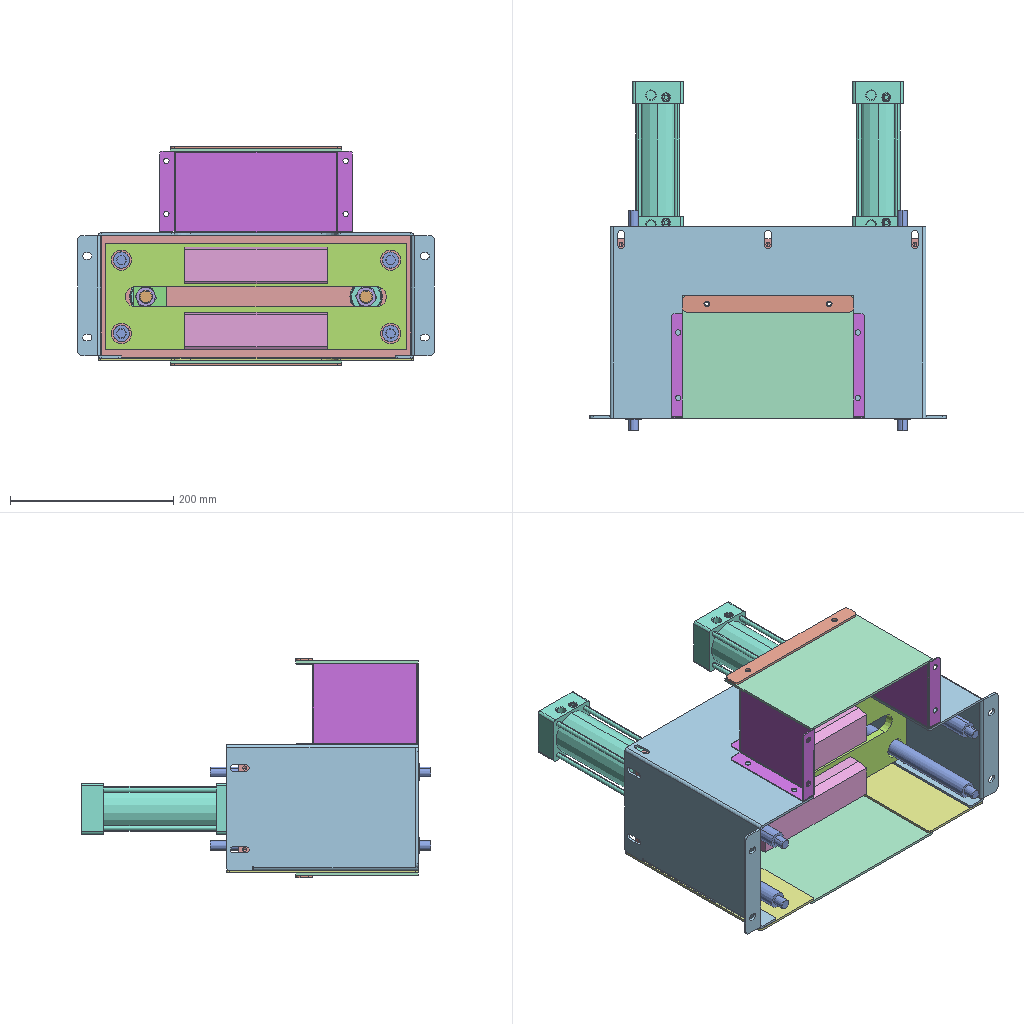Assembly | SolidWorks | 15 different items | 25 placed | box 437 x 428 x 269 mm
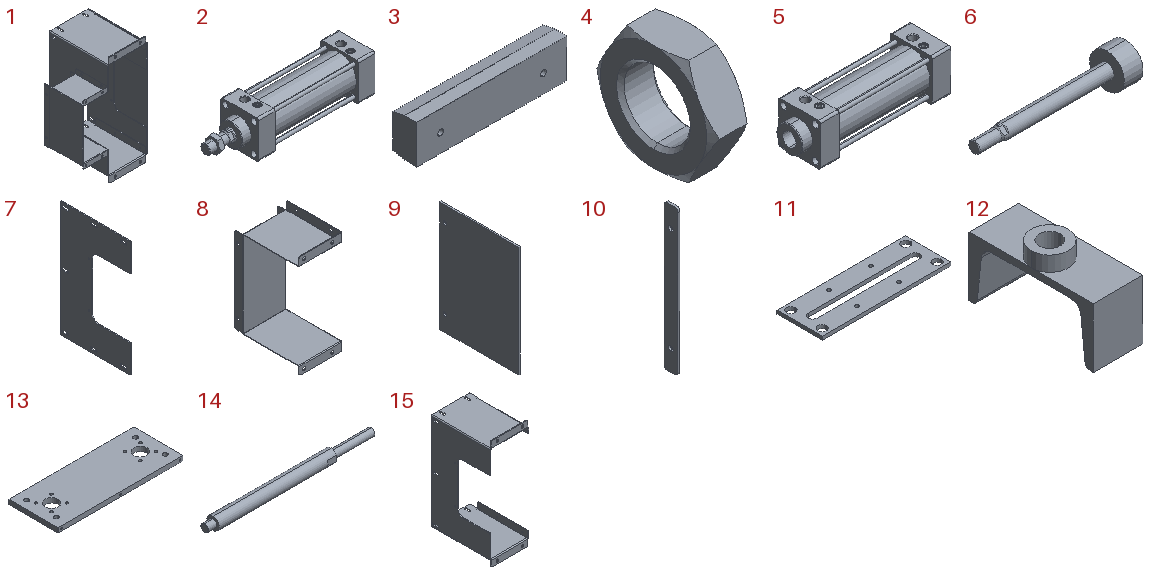Parts list (item | name | quantity | parent item | size | volume | features):
1 | (subassembly) | x1 | - | 269 x 235 x 437 mm | 927122 mm3 | features AEMSimFeature 1
2 | (subassembly) | x2 | - | 250 x 62 x 62 mm | 379695 mm3 | -
3 | - | x2 | - | 175 x 28 x 45 mm | 211666 mm3 | features Extrusion 1, HoleWzd 1, ICE 1
4 | - | x2 | in 2 | 8 x 26.558 x 23 mm | 2309 mm3 | features BaseBody 1
5 | - | x2 | in 2 | 208 x 62 x 62 mm | 269760 mm3 | features BaseBody 1
6 | - | x2 | in 2 | 217 x 49.5 x 49.5 mm | 107628 mm3 | features BaseBody 1
7 | - | x1 | in 1 | 3 x 235 x 387 mm | 191622 mm3 | features Fillet 3, FlatPattern 1, HoleWzd 1, ICE 1, SMBaseFlange 1, SheetMetal 1
8 | - | x1 | in 1 | 100 x 148.8 x 237.6 mm | 72757 mm3 | features HoleWzd 3, EdgeFlange 2, Fillet 2, FlatPattern 1, SMBaseFlange 1, SheetMetal 1
9 | - | x2 | in 1 | 3 x 150 x 210 mm | 94269 mm3 | features FlatPattern 1, HoleWzd 1, SMBaseFlange 1, SheetMetal 1
10 | - | x2 | in 1 | 3 x 20 x 210 mm | 12305 mm3 | features Fillet 1, FlatPattern 1, HoleWzd 1, SMBaseFlange 1, SheetMetal 1
11 | - | x1 | - | 370 x 130 x 10 mm | 379565 mm3 | features Extrusion 1, HoleWzd 1
12 | - | x1 | - | 40 x 100 x 60 mm | 55523 mm3 | features ICE 2, 3DProfileFeature 1, WeldMemberFeat 1, WeldmentFeature 1
13 | - | x1 | - | 380 x 150 x 14 mm | 746680 mm3 | features HoleWzd 6, 3DProfileFeature 2, Chamfer 1, Extrusion 1, ICE 1, LPattern 1
14 | - | x4 | - | 270 x 20 x 20 mm | 68758 mm3 | features ICE 2, Chamfer 1, Revolution 1
15 | - | x1 | in 1 | 154 x 235 x 437 mm | 449596 mm3 | features Fillet 4, ICE 4, EdgeFlange 3, HoleWzd 2, Cut 1, FlatPattern 1, SMBaseFlange 1, SheetMetal 1
Mates (type | each side: item.copy, entity, surface, feature):
In the top assembly
Coincident | 13.1 face plane Boss-Extrude1 | assembly face
Concentric | 13.1 face cylinder Cut-Extrude1 | assembly face
Concentric | 13.1 face cylinder Ø8.0 (8) Diameter Hole1 | assembly face
Concentric | assembly face | assembly face
LimitDistanceDim | assembly face | assembly face
Concentric | 13.1 face cylinder Ø13.0 (13) Diameter Hole1 | 14.1 face cylinder Revolve1
DistanceDim | 13.1 face plane Boss-Extrude1 | 14.1 face plane Revolve1
Coincident | 14.1 face plane Revolve1 | 14.2 face plane Revolve1 | 2 times
Coincident | 14.1 face plane Revolve1 | 14.3 face plane Revolve1 | 2 times
Coincident | 14.4 face plane Revolve1 | 14.3 face plane Revolve1 | 2 times
Concentric | 14.1 face cylinder Revolve1 | 11.1 face cylinder Boss-Extrude1
Concentric | 14.4 face cylinder Revolve1 | 11.1 face cylinder Boss-Extrude1
Concentric | 13.1 face cylinder Ø13.0 (13) Diameter Hole1 | 14.4 face cylinder Revolve1
Concentric | 13.1 face cylinder Ø13.0 (13) Diameter Hole1 | 14.3 face cylinder Revolve1
Concentric | 13.1 face cylinder Ø13.0 (13) Diameter Hole1 | 14.2 face cylinder Revolve1
Concentric | 11.1 face cylinder M8 Clearance Hole1 | 3.1 face cylinder M8 Tapped Hole1 | 2 times
Concentric | 11.1 face cylinder M8 Clearance Hole1 | 3.2 face cylinder M8 Tapped Hole1 | 2 times
Coincident | 11.1 face plane Boss-Extrude1 | 3.2 face plane Boss-Extrude1
Coincident | 11.1 face plane Boss-Extrude1 | 3.1 face plane Boss-Extrude1
Coincident | 13.1 face plane Boss-Extrude1 | 5.1 face plane Import1
Concentric | 13.1 face cylinder Cut-Extrude1 | 6.1 face cylinder Import1
DistanceDim | 13.1 face plane Boss-Extrude1 | 11.1 face plane Boss-Extrude1
Concentric | 6.1 face cylinder Import1 | 12.1 face cylinder Cut-Extrude1
DistanceDim | 13.1 face plane Boss-Extrude1 | 15.1 face plane Base-Flange1
DistanceDim | 15.1 face plane Edge-Flange1 | 13.1 face plane Boss-Extrude1
DistanceDim | 15.1 face plane Edge-Flange3 | 14.4 face plane Revolve1
In subassembly 2
LimitDistanceDim | 6.2 face plane Import1 | 5.2 face plane Import1
Concentric | 5.2 face cylinder Import1 | 6.2 face cylinder Import1
DistanceDim | 6.2 face plane Import1 | 4.1 face plane Import1
Concentric | 6.2 face cylinder Import1 | 4.1 face cylinder Import1
In subassembly 1
Coincident | 15.2 face plane Edge-Flange2 | 7.1 face plane Base-Flange1
Coincident | 15.2 face plane Edge-Flange1 | 7.1 face plane Base-Flange1 | 2 times
Coincident | 15.2 face plane Base-Flange1 | 8.1 face plane Edge-Flange1 | 2 times
Width | 15.2 face plane Edge-Flange1 | 15.2 face plane Edge-Flange1 | 8.1 face plane Base-Flange1 | 8.1 face plane Base-Flange1
Coincident | 9.1 face plane Base-Flange1 | 8.1 face plane Edge-Flange2
Coincident | 9.1 face plane Base-Flange1 | 8.1 face plane Edge-Flange1
Width | 9.1 face plane Base-Flange1 | 9.1 face plane Base-Flange1 | 8.1 face plane Base-Flange1 | 8.1 face plane Base-Flange1
Coincident | 7.1 face plane Base-Flange1 | 9.2 face plane Base-Flange1
Coincident | 9.1 face plane Base-Flange1 | 9.2 face plane Base-Flange1 | 2 times
Concentric | 9.1 face cylinder M6 Clearance Hole1 | 10.1 face cylinder M6 Clearance Hole1
Coincident | 9.1 face plane Base-Flange1 | 10.1 face plane Base-Flange1
Coincident | 9.2 face plane Base-Flange1 | 10.2 face plane Base-Flange1
Concentric | 9.2 face cylinder M6 Clearance Hole1 | 10.2 face cylinder M6 Clearance Hole1